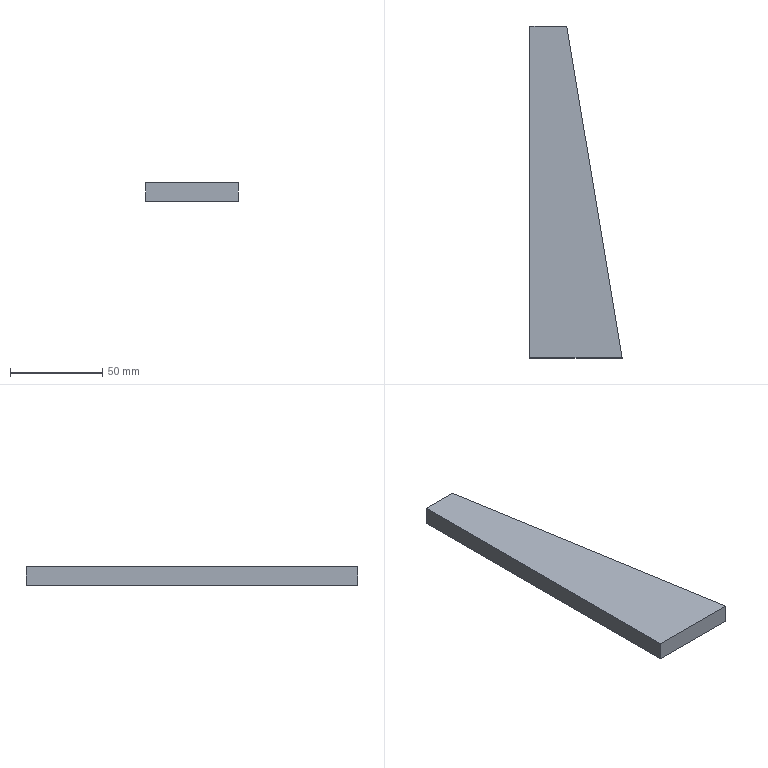Part | STEP file | Traction motor rib plate QY-2-03 | 1 solid | 6 faces | box 50 x 180 x 10 mm | volume 63000 mm3 | plane 6
STEP:
#1=CARTESIAN_POINT('',(0.,0.,0.));
#2=DIRECTION('',(0.,0.,1.));
#3=DIRECTION('',(1.,0.,0.));
#4=AXIS2_PLACEMENT_3D('',#1,#2,#3);
#5=CARTESIAN_POINT('',(0.,0.,0.));
#6=VERTEX_POINT('',#5);
#7=CARTESIAN_POINT('',(50.,0.,0.));
#8=VERTEX_POINT('',#7);
#9=CARTESIAN_POINT('',(50.,0.,0.));
#10=DIRECTION('',(1.,0.,0.));
#11=VECTOR('',#10,1.);
#12=LINE('',#9,#11);
#13=CARTESIAN_POINT('',(50.,0.,10.));
#14=DIRECTION('',(0.,1.,0.));
#15=DIRECTION('',(0.,0.,1.));
#16=AXIS2_PLACEMENT_3D('',#13,#14,#15);
#17=PLANE('',#16);
#18=CARTESIAN_POINT('',(-10.,0.));
#19=DIRECTION('',(0.,1.));
#20=VECTOR('',#19,1.);
#21=LINE('',#18,#20);
#22=(GEOMETRIC_REPRESENTATION_CONTEXT(2)PARAMETRIC_REPRESENTATION_CONTEXT()REPRESENTATION_CONTEXT('',''));
#23=DEFINITIONAL_REPRESENTATION('',(#21),#22);
#24=PCURVE('',#17,#23);
#25=CARTESIAN_POINT('',(0.,0.,0.));
#26=DIRECTION('',(0.,0.,-1.));
#27=DIRECTION('',(-1.,0.,0.));
#28=AXIS2_PLACEMENT_3D('',#25,#26,#27);
#29=PLANE('',#28);
#30=CARTESIAN_POINT('',(-50.,0.));
#31=DIRECTION('',(-1.,0.));
#32=VECTOR('',#31,1.);
#33=LINE('',#30,#32);
#34=(GEOMETRIC_REPRESENTATION_CONTEXT(2)PARAMETRIC_REPRESENTATION_CONTEXT()REPRESENTATION_CONTEXT('',''));
#35=DEFINITIONAL_REPRESENTATION('',(#33),#34);
#36=PCURVE('',#29,#35);
#37=SURFACE_CURVE('',#12,(#24,#36),.PCURVE_S1.);
#38=EDGE_CURVE('',#6,#8,#37,.T.);
#39=ORIENTED_EDGE('',*,*,#38,.T.);
#40=CARTESIAN_POINT('',(50.,0.,10.));
#41=VERTEX_POINT('',#40);
#42=CARTESIAN_POINT('',(50.,0.,10.));
#43=DIRECTION('',(0.,0.,-1.));
#44=VECTOR('',#43,1.);
#45=LINE('',#42,#44);
#46=CARTESIAN_POINT('',(0.,0.));
#47=DIRECTION('',(-1.,0.));
#48=VECTOR('',#47,1.);
#49=LINE('',#46,#48);
#50=(GEOMETRIC_REPRESENTATION_CONTEXT(2)PARAMETRIC_REPRESENTATION_CONTEXT()REPRESENTATION_CONTEXT('',''));
#51=DEFINITIONAL_REPRESENTATION('',(#49),#50);
#52=PCURVE('',#17,#51);
#53=CARTESIAN_POINT('',(20.,180.,10.));
#54=DIRECTION('',(-0.9864,-0.1644,0.));
#55=DIRECTION('',(0.1644,-0.9864,0.));
#56=AXIS2_PLACEMENT_3D('',#53,#54,#55);
#57=PLANE('',#56);
#58=CARTESIAN_POINT('',(182.483,0.));
#59=DIRECTION('',(0.,-1.));
#60=VECTOR('',#59,1.);
#61=LINE('',#58,#60);
#62=(GEOMETRIC_REPRESENTATION_CONTEXT(2)PARAMETRIC_REPRESENTATION_CONTEXT()REPRESENTATION_CONTEXT('',''));
#63=DEFINITIONAL_REPRESENTATION('',(#61),#62);
#64=PCURVE('',#57,#63);
#65=SURFACE_CURVE('',#45,(#52,#64),.PCURVE_S1.);
#66=EDGE_CURVE('',#41,#8,#65,.T.);
#67=ORIENTED_EDGE('',*,*,#66,.F.);
#68=CARTESIAN_POINT('',(0.,0.,10.));
#69=VERTEX_POINT('',#68);
#70=CARTESIAN_POINT('',(50.,0.,10.));
#71=DIRECTION('',(1.,0.,0.));
#72=VECTOR('',#71,1.);
#73=LINE('',#70,#72);
#74=CARTESIAN_POINT('',(0.,0.));
#75=DIRECTION('',(0.,1.));
#76=VECTOR('',#75,1.);
#77=LINE('',#74,#76);
#78=(GEOMETRIC_REPRESENTATION_CONTEXT(2)PARAMETRIC_REPRESENTATION_CONTEXT()REPRESENTATION_CONTEXT('',''));
#79=DEFINITIONAL_REPRESENTATION('',(#77),#78);
#80=PCURVE('',#17,#79);
#81=CARTESIAN_POINT('',(0.,0.,10.));
#82=DIRECTION('',(0.,0.,-1.));
#83=DIRECTION('',(-1.,0.,0.));
#84=AXIS2_PLACEMENT_3D('',#81,#82,#83);
#85=PLANE('',#84);
#86=CARTESIAN_POINT('',(-50.,0.));
#87=DIRECTION('',(-1.,0.));
#88=VECTOR('',#87,1.);
#89=LINE('',#86,#88);
#90=(GEOMETRIC_REPRESENTATION_CONTEXT(2)PARAMETRIC_REPRESENTATION_CONTEXT()REPRESENTATION_CONTEXT('',''));
#91=DEFINITIONAL_REPRESENTATION('',(#89),#90);
#92=PCURVE('',#85,#91);
#93=SURFACE_CURVE('',#73,(#80,#92),.PCURVE_S1.);
#94=EDGE_CURVE('',#69,#41,#93,.T.);
#95=ORIENTED_EDGE('',*,*,#94,.F.);
#96=CARTESIAN_POINT('',(0.,0.,10.));
#97=DIRECTION('',(0.,0.,-1.));
#98=VECTOR('',#97,1.);
#99=LINE('',#96,#98);
#100=CARTESIAN_POINT('',(0.,-50.));
#101=DIRECTION('',(-1.,0.));
#102=VECTOR('',#101,1.);
#103=LINE('',#100,#102);
#104=(GEOMETRIC_REPRESENTATION_CONTEXT(2)PARAMETRIC_REPRESENTATION_CONTEXT()REPRESENTATION_CONTEXT('',''));
#105=DEFINITIONAL_REPRESENTATION('',(#103),#104);
#106=PCURVE('',#17,#105);
#107=CARTESIAN_POINT('',(0.,0.,10.));
#108=DIRECTION('',(1.,0.,0.));
#109=DIRECTION('',(0.,0.,-1.));
#110=AXIS2_PLACEMENT_3D('',#107,#108,#109);
#111=PLANE('',#110);
#112=CARTESIAN_POINT('',(0.,0.));
#113=DIRECTION('',(1.,0.));
#114=VECTOR('',#113,1.);
#115=LINE('',#112,#114);
#116=(GEOMETRIC_REPRESENTATION_CONTEXT(2)PARAMETRIC_REPRESENTATION_CONTEXT()REPRESENTATION_CONTEXT('',''));
#117=DEFINITIONAL_REPRESENTATION('',(#115),#116);
#118=PCURVE('',#111,#117);
#119=SURFACE_CURVE('',#99,(#106,#118),.PCURVE_S1.);
#120=EDGE_CURVE('',#69,#6,#119,.T.);
#121=ORIENTED_EDGE('',*,*,#120,.T.);
#122=EDGE_LOOP('',(#39,#67,#95,#121));
#123=FACE_BOUND('',#122,.T.);
#124=ADVANCED_FACE('',(#123),#17,.F.);
#125=CARTESIAN_POINT('',(20.,180.,0.));
#126=VERTEX_POINT('',#125);
#127=CARTESIAN_POINT('',(20.,180.,0.));
#128=DIRECTION('',(-0.1644,0.9864,0.));
#129=VECTOR('',#128,1.);
#130=LINE('',#127,#129);
#131=CARTESIAN_POINT('',(0.,-10.));
#132=DIRECTION('',(-1.,0.));
#133=VECTOR('',#132,1.);
#134=LINE('',#131,#133);
#135=(GEOMETRIC_REPRESENTATION_CONTEXT(2)PARAMETRIC_REPRESENTATION_CONTEXT()REPRESENTATION_CONTEXT('',''));
#136=DEFINITIONAL_REPRESENTATION('',(#134),#135);
#137=PCURVE('',#57,#136);
#138=CARTESIAN_POINT('',(-20.,180.));
#139=DIRECTION('',(0.1644,0.9864));
#140=VECTOR('',#139,1.);
#141=LINE('',#138,#140);
#142=(GEOMETRIC_REPRESENTATION_CONTEXT(2)PARAMETRIC_REPRESENTATION_CONTEXT()REPRESENTATION_CONTEXT('',''));
#143=DEFINITIONAL_REPRESENTATION('',(#141),#142);
#144=PCURVE('',#29,#143);
#145=SURFACE_CURVE('',#130,(#137,#144),.PCURVE_S1.);
#146=EDGE_CURVE('',#8,#126,#145,.T.);
#147=ORIENTED_EDGE('',*,*,#146,.T.);
#148=CARTESIAN_POINT('',(20.,180.,10.));
#149=VERTEX_POINT('',#148);
#150=CARTESIAN_POINT('',(20.,180.,10.));
#151=DIRECTION('',(0.,0.,-1.));
#152=VECTOR('',#151,1.);
#153=LINE('',#150,#152);
#154=CARTESIAN_POINT('',(0.,0.));
#155=DIRECTION('',(0.,-1.));
#156=VECTOR('',#155,1.);
#157=LINE('',#154,#156);
#158=(GEOMETRIC_REPRESENTATION_CONTEXT(2)PARAMETRIC_REPRESENTATION_CONTEXT()REPRESENTATION_CONTEXT('',''));
#159=DEFINITIONAL_REPRESENTATION('',(#157),#158);
#160=PCURVE('',#57,#159);
#161=CARTESIAN_POINT('',(0.,180.,10.));
#162=DIRECTION('',(0.,-1.,0.));
#163=DIRECTION('',(0.,0.,-1.));
#164=AXIS2_PLACEMENT_3D('',#161,#162,#163);
#165=PLANE('',#164);
#166=CARTESIAN_POINT('',(0.,20.));
#167=DIRECTION('',(1.,0.));
#168=VECTOR('',#167,1.);
#169=LINE('',#166,#168);
#170=(GEOMETRIC_REPRESENTATION_CONTEXT(2)PARAMETRIC_REPRESENTATION_CONTEXT()REPRESENTATION_CONTEXT('',''));
#171=DEFINITIONAL_REPRESENTATION('',(#169),#170);
#172=PCURVE('',#165,#171);
#173=SURFACE_CURVE('',#153,(#160,#172),.PCURVE_S1.);
#174=EDGE_CURVE('',#149,#126,#173,.T.);
#175=ORIENTED_EDGE('',*,*,#174,.F.);
#176=CARTESIAN_POINT('',(20.,180.,10.));
#177=DIRECTION('',(-0.1644,0.9864,0.));
#178=VECTOR('',#177,1.);
#179=LINE('',#176,#178);
#180=CARTESIAN_POINT('',(0.,0.));
#181=DIRECTION('',(-1.,0.));
#182=VECTOR('',#181,1.);
#183=LINE('',#180,#182);
#184=(GEOMETRIC_REPRESENTATION_CONTEXT(2)PARAMETRIC_REPRESENTATION_CONTEXT()REPRESENTATION_CONTEXT('',''));
#185=DEFINITIONAL_REPRESENTATION('',(#183),#184);
#186=PCURVE('',#57,#185);
#187=CARTESIAN_POINT('',(-20.,180.));
#188=DIRECTION('',(0.1644,0.9864));
#189=VECTOR('',#188,1.);
#190=LINE('',#187,#189);
#191=(GEOMETRIC_REPRESENTATION_CONTEXT(2)PARAMETRIC_REPRESENTATION_CONTEXT()REPRESENTATION_CONTEXT('',''));
#192=DEFINITIONAL_REPRESENTATION('',(#190),#191);
#193=PCURVE('',#85,#192);
#194=SURFACE_CURVE('',#179,(#186,#193),.PCURVE_S1.);
#195=EDGE_CURVE('',#41,#149,#194,.T.);
#196=ORIENTED_EDGE('',*,*,#195,.F.);
#197=ORIENTED_EDGE('',*,*,#66,.T.);
#198=EDGE_LOOP('',(#147,#175,#196,#197));
#199=FACE_BOUND('',#198,.T.);
#200=ADVANCED_FACE('',(#199),#57,.F.);
#201=CARTESIAN_POINT('',(0.,180.,0.));
#202=VERTEX_POINT('',#201);
#203=CARTESIAN_POINT('',(0.,180.,0.));
#204=DIRECTION('',(-1.,0.,0.));
#205=VECTOR('',#204,1.);
#206=LINE('',#203,#205);
#207=CARTESIAN_POINT('',(10.,0.));
#208=DIRECTION('',(0.,-1.));
#209=VECTOR('',#208,1.);
#210=LINE('',#207,#209);
#211=(GEOMETRIC_REPRESENTATION_CONTEXT(2)PARAMETRIC_REPRESENTATION_CONTEXT()REPRESENTATION_CONTEXT('',''));
#212=DEFINITIONAL_REPRESENTATION('',(#210),#211);
#213=PCURVE('',#165,#212);
#214=CARTESIAN_POINT('',(0.,180.));
#215=DIRECTION('',(1.,0.));
#216=VECTOR('',#215,1.);
#217=LINE('',#214,#216);
#218=(GEOMETRIC_REPRESENTATION_CONTEXT(2)PARAMETRIC_REPRESENTATION_CONTEXT()REPRESENTATION_CONTEXT('',''));
#219=DEFINITIONAL_REPRESENTATION('',(#217),#218);
#220=PCURVE('',#29,#219);
#221=SURFACE_CURVE('',#206,(#213,#220),.PCURVE_S1.);
#222=EDGE_CURVE('',#126,#202,#221,.T.);
#223=ORIENTED_EDGE('',*,*,#222,.T.);
#224=CARTESIAN_POINT('',(0.,180.,10.));
#225=VERTEX_POINT('',#224);
#226=CARTESIAN_POINT('',(0.,180.,10.));
#227=DIRECTION('',(0.,0.,-1.));
#228=VECTOR('',#227,1.);
#229=LINE('',#226,#228);
#230=CARTESIAN_POINT('',(0.,0.));
#231=DIRECTION('',(1.,0.));
#232=VECTOR('',#231,1.);
#233=LINE('',#230,#232);
#234=(GEOMETRIC_REPRESENTATION_CONTEXT(2)PARAMETRIC_REPRESENTATION_CONTEXT()REPRESENTATION_CONTEXT('',''));
#235=DEFINITIONAL_REPRESENTATION('',(#233),#234);
#236=PCURVE('',#165,#235);
#237=CARTESIAN_POINT('',(0.,180.));
#238=DIRECTION('',(1.,0.));
#239=VECTOR('',#238,1.);
#240=LINE('',#237,#239);
#241=(GEOMETRIC_REPRESENTATION_CONTEXT(2)PARAMETRIC_REPRESENTATION_CONTEXT()REPRESENTATION_CONTEXT('',''));
#242=DEFINITIONAL_REPRESENTATION('',(#240),#241);
#243=PCURVE('',#111,#242);
#244=SURFACE_CURVE('',#229,(#236,#243),.PCURVE_S1.);
#245=EDGE_CURVE('',#225,#202,#244,.T.);
#246=ORIENTED_EDGE('',*,*,#245,.F.);
#247=CARTESIAN_POINT('',(0.,180.,10.));
#248=DIRECTION('',(-1.,0.,0.));
#249=VECTOR('',#248,1.);
#250=LINE('',#247,#249);
#251=CARTESIAN_POINT('',(0.,0.));
#252=DIRECTION('',(0.,-1.));
#253=VECTOR('',#252,1.);
#254=LINE('',#251,#253);
#255=(GEOMETRIC_REPRESENTATION_CONTEXT(2)PARAMETRIC_REPRESENTATION_CONTEXT()REPRESENTATION_CONTEXT('',''));
#256=DEFINITIONAL_REPRESENTATION('',(#254),#255);
#257=PCURVE('',#165,#256);
#258=CARTESIAN_POINT('',(0.,180.));
#259=DIRECTION('',(1.,0.));
#260=VECTOR('',#259,1.);
#261=LINE('',#258,#260);
#262=(GEOMETRIC_REPRESENTATION_CONTEXT(2)PARAMETRIC_REPRESENTATION_CONTEXT()REPRESENTATION_CONTEXT('',''));
#263=DEFINITIONAL_REPRESENTATION('',(#261),#262);
#264=PCURVE('',#85,#263);
#265=SURFACE_CURVE('',#250,(#257,#264),.PCURVE_S1.);
#266=EDGE_CURVE('',#149,#225,#265,.T.);
#267=ORIENTED_EDGE('',*,*,#266,.F.);
#268=ORIENTED_EDGE('',*,*,#174,.T.);
#269=EDGE_LOOP('',(#223,#246,#267,#268));
#270=FACE_BOUND('',#269,.T.);
#271=ADVANCED_FACE('',(#270),#165,.F.);
#272=CARTESIAN_POINT('',(0.,0.,0.));
#273=DIRECTION('',(0.,-1.,0.));
#274=VECTOR('',#273,1.);
#275=LINE('',#272,#274);
#276=CARTESIAN_POINT('',(10.,0.));
#277=DIRECTION('',(0.,-1.));
#278=VECTOR('',#277,1.);
#279=LINE('',#276,#278);
#280=(GEOMETRIC_REPRESENTATION_CONTEXT(2)PARAMETRIC_REPRESENTATION_CONTEXT()REPRESENTATION_CONTEXT('',''));
#281=DEFINITIONAL_REPRESENTATION('',(#279),#280);
#282=PCURVE('',#111,#281);
#283=CARTESIAN_POINT('',(0.,0.));
#284=DIRECTION('',(0.,-1.));
#285=VECTOR('',#284,1.);
#286=LINE('',#283,#285);
#287=(GEOMETRIC_REPRESENTATION_CONTEXT(2)PARAMETRIC_REPRESENTATION_CONTEXT()REPRESENTATION_CONTEXT('',''));
#288=DEFINITIONAL_REPRESENTATION('',(#286),#287);
#289=PCURVE('',#29,#288);
#290=SURFACE_CURVE('',#275,(#282,#289),.PCURVE_S1.);
#291=EDGE_CURVE('',#202,#6,#290,.T.);
#292=ORIENTED_EDGE('',*,*,#291,.T.);
#293=ORIENTED_EDGE('',*,*,#120,.F.);
#294=CARTESIAN_POINT('',(0.,0.,10.));
#295=DIRECTION('',(0.,-1.,0.));
#296=VECTOR('',#295,1.);
#297=LINE('',#294,#296);
#298=CARTESIAN_POINT('',(0.,0.));
#299=DIRECTION('',(0.,-1.));
#300=VECTOR('',#299,1.);
#301=LINE('',#298,#300);
#302=(GEOMETRIC_REPRESENTATION_CONTEXT(2)PARAMETRIC_REPRESENTATION_CONTEXT()REPRESENTATION_CONTEXT('',''));
#303=DEFINITIONAL_REPRESENTATION('',(#301),#302);
#304=PCURVE('',#111,#303);
#305=CARTESIAN_POINT('',(0.,0.));
#306=DIRECTION('',(0.,-1.));
#307=VECTOR('',#306,1.);
#308=LINE('',#305,#307);
#309=(GEOMETRIC_REPRESENTATION_CONTEXT(2)PARAMETRIC_REPRESENTATION_CONTEXT()REPRESENTATION_CONTEXT('',''));
#310=DEFINITIONAL_REPRESENTATION('',(#308),#309);
#311=PCURVE('',#85,#310);
#312=SURFACE_CURVE('',#297,(#304,#311),.PCURVE_S1.);
#313=EDGE_CURVE('',#225,#69,#312,.T.);
#314=ORIENTED_EDGE('',*,*,#313,.F.);
#315=ORIENTED_EDGE('',*,*,#245,.T.);
#316=EDGE_LOOP('',(#292,#293,#314,#315));
#317=FACE_BOUND('',#316,.T.);
#318=ADVANCED_FACE('',(#317),#111,.F.);
#319=ORIENTED_EDGE('',*,*,#94,.T.);
#320=ORIENTED_EDGE('',*,*,#195,.T.);
#321=ORIENTED_EDGE('',*,*,#266,.T.);
#322=ORIENTED_EDGE('',*,*,#313,.T.);
#323=EDGE_LOOP('',(#319,#320,#321,#322));
#324=FACE_BOUND('',#323,.T.);
#325=ADVANCED_FACE('',(#324),#85,.F.);
#326=ORIENTED_EDGE('',*,*,#38,.F.);
#327=ORIENTED_EDGE('',*,*,#291,.F.);
#328=ORIENTED_EDGE('',*,*,#222,.F.);
#329=ORIENTED_EDGE('',*,*,#146,.F.);
#330=EDGE_LOOP('',(#326,#327,#328,#329));
#331=FACE_BOUND('',#330,.T.);
#332=ADVANCED_FACE('',(#331),#29,.T.);
#333=CLOSED_SHELL('',(#124,#200,#271,#318,#325,#332));
#334=MANIFOLD_SOLID_BREP('',#333);
#335=(LENGTH_UNIT()NAMED_UNIT(*)SI_UNIT(.MILLI.,.METRE.));
#336=UNCERTAINTY_MEASURE_WITH_UNIT(LENGTH_MEASURE(0.0000001),#335,'','');
#337=(NAMED_UNIT(*)PLANE_ANGLE_UNIT()SI_UNIT($,.RADIAN.));
#338=(NAMED_UNIT(*)SI_UNIT($,.STERADIAN.)SOLID_ANGLE_UNIT());
#339=(GEOMETRIC_REPRESENTATION_CONTEXT(3)GLOBAL_UNCERTAINTY_ASSIGNED_CONTEXT((#336))GLOBAL_UNIT_ASSIGNED_CONTEXT((#335,#337,#338))REPRESENTATION_CONTEXT('',''));
#340=ADVANCED_BREP_SHAPE_REPRESENTATION('',(#4,#334),#339);